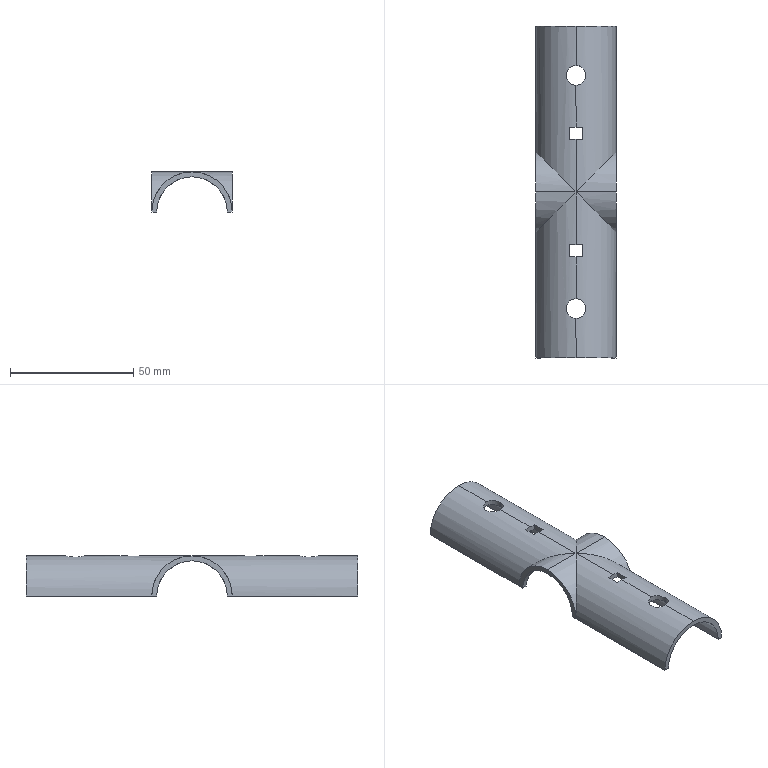Part | STEP file | F-B | 1 solid | 36 faces | box 32.6 x 134.6 x 16.3 mm | volume 12017 mm3 | cylinder 20 | plane 16 | commonest cylinder face diameters 28.6 x8 32.6 x8 8 x4